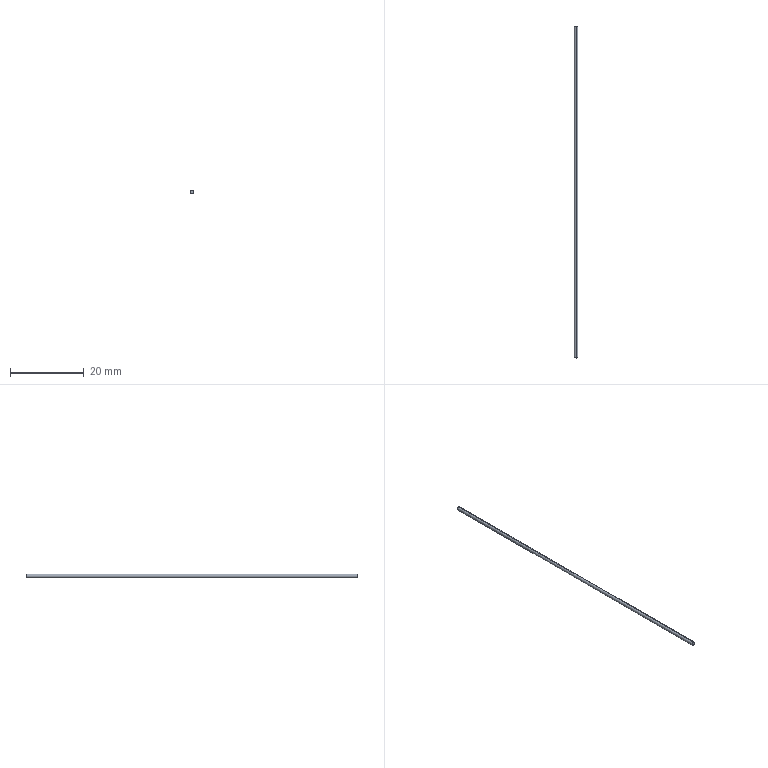Part | SolidWorks | features Revolution 1 | 1 solid | 4 faces | box 1 x 90 x 1 mm | volume 70.686 mm3 | cylinder 2 | plane 2 | commonest cylinder face diameters 1 x2
STEP:
#1=CARTESIAN_POINT('',(0.,90.,-0.5));
#2=VERTEX_POINT('',#1);
#3=CARTESIAN_POINT('',(0.,90.,0.5));
#4=VERTEX_POINT('',#3);
#5=CARTESIAN_POINT('',(0.,90.,0.));
#6=DIRECTION('',(0.,-1.,0.));
#7=DIRECTION('',(0.,0.,-1.));
#8=AXIS2_PLACEMENT_3D('',#5,#6,#7);
#9=CIRCLE('',#8,0.5);
#10=EDGE_CURVE('',#2,#4,#9,.T.);
#11=ORIENTED_EDGE('',*,*,#10,.T.);
#12=CARTESIAN_POINT('',(0.,0.,0.5));
#13=VERTEX_POINT('',#12);
#14=CARTESIAN_POINT('',(0.,-6.442,0.5));
#15=DIRECTION('',(0.,-1.,0.));
#16=VECTOR('',#15,1000.);
#17=LINE('',#14,#16);
#18=EDGE_CURVE('',#4,#13,#17,.T.);
#19=ORIENTED_EDGE('',*,*,#18,.T.);
#20=CARTESIAN_POINT('',(0.,0.,-0.5));
#21=VERTEX_POINT('',#20);
#22=CARTESIAN_POINT('',(0.,0.,0.));
#23=DIRECTION('',(0.,-1.,0.));
#24=DIRECTION('',(0.,0.,-1.));
#25=AXIS2_PLACEMENT_3D('',#22,#23,#24);
#26=CIRCLE('',#25,0.5);
#27=EDGE_CURVE('',#21,#13,#26,.T.);
#28=ORIENTED_EDGE('',*,*,#27,.F.);
#29=CARTESIAN_POINT('',(0.,-6.442,-0.5));
#30=DIRECTION('',(0.,-1.,0.));
#31=VECTOR('',#30,1000.);
#32=LINE('',#29,#31);
#33=EDGE_CURVE('',#2,#21,#32,.T.);
#34=ORIENTED_EDGE('',*,*,#33,.F.);
#35=EDGE_LOOP('',(#11,#19,#28,#34));
#36=FACE_OUTER_BOUND('',#35,.T.);
#37=CARTESIAN_POINT('',(0.,-6.442,0.));
#38=DIRECTION('',(0.,-1.,0.));
#39=DIRECTION('',(0.,0.,-1.));
#40=AXIS2_PLACEMENT_3D('',#37,#38,#39);
#41=CYLINDRICAL_SURFACE('',#40,0.5);
#42=ADVANCED_FACE('',(#36),#41,.T.);
#43=ORIENTED_EDGE('',*,*,#10,.F.);
#44=CARTESIAN_POINT('',(0.,90.,0.));
#45=DIRECTION('',(0.,-1.,0.));
#46=DIRECTION('',(0.,0.,-1.));
#47=AXIS2_PLACEMENT_3D('',#44,#45,#46);
#48=CIRCLE('',#47,0.5);
#49=EDGE_CURVE('',#4,#2,#48,.T.);
#50=ORIENTED_EDGE('',*,*,#49,.F.);
#51=EDGE_LOOP('',(#43,#50));
#52=FACE_OUTER_BOUND('',#51,.T.);
#53=CARTESIAN_POINT('',(0.,90.,0.));
#54=DIRECTION('',(0.,-1.,0.));
#55=DIRECTION('',(0.,0.,-1.));
#56=AXIS2_PLACEMENT_3D('',#53,#54,#55);
#57=PLANE('',#56);
#58=ADVANCED_FACE('',(#52),#57,.F.);
#59=ORIENTED_EDGE('',*,*,#18,.F.);
#60=ORIENTED_EDGE('',*,*,#49,.T.);
#61=ORIENTED_EDGE('',*,*,#33,.T.);
#62=CARTESIAN_POINT('',(0.,0.,0.));
#63=DIRECTION('',(0.,-1.,0.));
#64=DIRECTION('',(0.,0.,-1.));
#65=AXIS2_PLACEMENT_3D('',#62,#63,#64);
#66=CIRCLE('',#65,0.5);
#67=EDGE_CURVE('',#13,#21,#66,.T.);
#68=ORIENTED_EDGE('',*,*,#67,.F.);
#69=EDGE_LOOP('',(#59,#60,#61,#68));
#70=FACE_OUTER_BOUND('',#69,.T.);
#71=CARTESIAN_POINT('',(0.,-6.442,0.));
#72=DIRECTION('',(0.,-1.,0.));
#73=DIRECTION('',(0.,0.,-1.));
#74=AXIS2_PLACEMENT_3D('',#71,#72,#73);
#75=CYLINDRICAL_SURFACE('',#74,0.5);
#76=ADVANCED_FACE('',(#70),#75,.T.);
#77=ORIENTED_EDGE('',*,*,#27,.T.);
#78=ORIENTED_EDGE('',*,*,#67,.T.);
#79=EDGE_LOOP('',(#77,#78));
#80=FACE_OUTER_BOUND('',#79,.T.);
#81=CARTESIAN_POINT('',(0.,0.,0.));
#82=DIRECTION('',(0.,1.,0.));
#83=DIRECTION('',(0.,0.,1.));
#84=AXIS2_PLACEMENT_3D('',#81,#82,#83);
#85=PLANE('',#84);
#86=ADVANCED_FACE('',(#80),#85,.F.);
#87=CLOSED_SHELL('',(#42,#58,#76,#86));
#88=MANIFOLD_SOLID_BREP('',#87);
#89=CARTESIAN_POINT('',(0.,0.,0.));
#90=DIRECTION('',(0.,0.,1.));
#91=DIRECTION('',(1.,0.,0.));
#92=AXIS2_PLACEMENT_3D('',#89,#90,#91);
#93=(LENGTH_UNIT()NAMED_UNIT(*)SI_UNIT(.MILLI.,.METRE.));
#94=UNCERTAINTY_MEASURE_WITH_UNIT(LENGTH_MEASURE(0.00001),#93,'','');
#95=(NAMED_UNIT(*)PLANE_ANGLE_UNIT()SI_UNIT($,.RADIAN.));
#96=(NAMED_UNIT(*)SI_UNIT($,.STERADIAN.)SOLID_ANGLE_UNIT());
#97=(GEOMETRIC_REPRESENTATION_CONTEXT(3)GLOBAL_UNCERTAINTY_ASSIGNED_CONTEXT((#94))GLOBAL_UNIT_ASSIGNED_CONTEXT((#93,#95,#96))REPRESENTATION_CONTEXT('',''));
#98=ADVANCED_BREP_SHAPE_REPRESENTATION('',(#88,#92),#97);